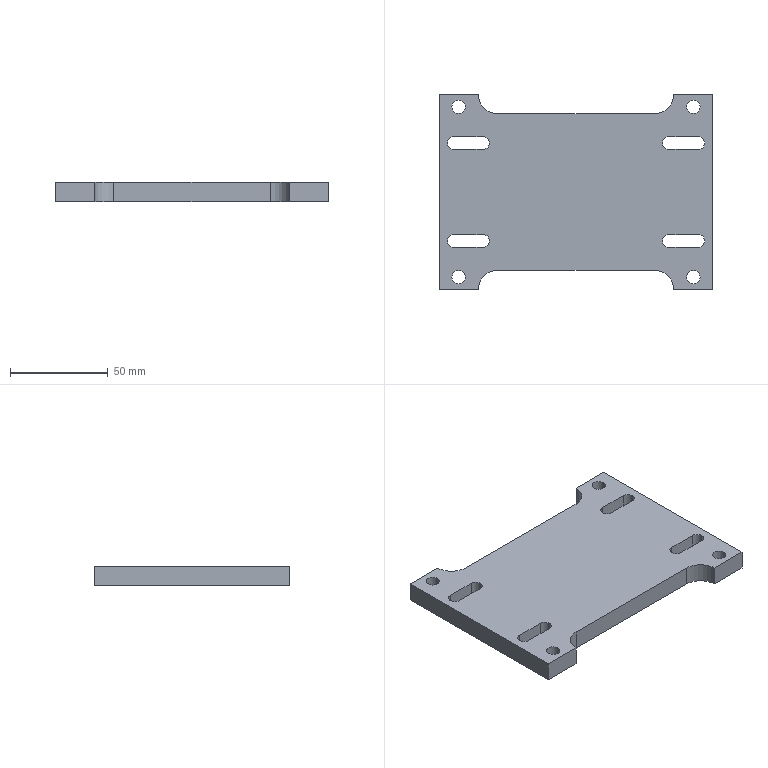Part | STEP file | B07 | 1 solid | 42 faces | box 140 x 100 x 10 mm | volume 114178 mm3 | cylinder 24 | plane 18 | commonest cylinder face diameters 6.5 x12 6.8 x8 20 x4